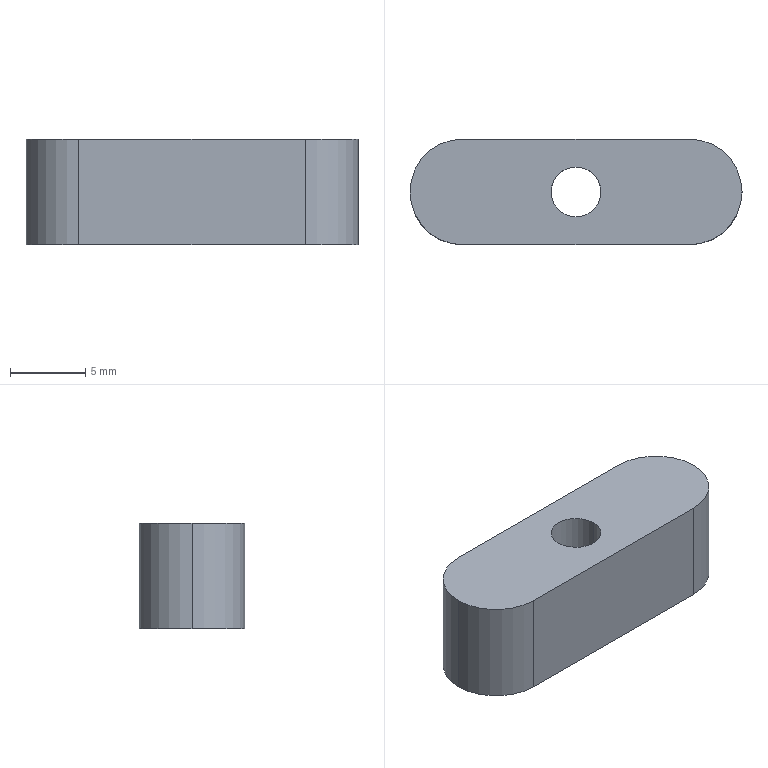Part | STEP file | BU-A13#130b | 1 solid | 9 faces | box 22 x 7 x 7 mm | volume 944.521 mm3 | cylinder 5 | plane 4 | commonest cylinder face diameters 7 x3 3.3 x2
STEP:
#1=CARTESIAN_POINT('',(0.,0.,0.));
#2=DIRECTION('',(0.,0.,1.));
#3=DIRECTION('',(1.,0.,0.));
#4=AXIS2_PLACEMENT_3D('',#1,#2,#3);
#5=CARTESIAN_POINT('',(9.15,0.,0.));
#6=VERTEX_POINT('',#5);
#7=CARTESIAN_POINT('',(9.15,0.,7.));
#8=VERTEX_POINT('',#7);
#9=CARTESIAN_POINT('',(9.15,0.,7.));
#10=DIRECTION('',(0.,0.,1.));
#11=VECTOR('',#10,1.);
#12=LINE('',#9,#11);
#13=CARTESIAN_POINT('',(7.5,0.,7.));
#14=DIRECTION('',(0.,0.,1.));
#15=DIRECTION('',(1.,0.,0.));
#16=AXIS2_PLACEMENT_3D('',#13,#14,#15);
#17=CYLINDRICAL_SURFACE('',#16,1.65);
#18=CARTESIAN_POINT('',(6.283,0.));
#19=DIRECTION('',(0.,1.));
#20=VECTOR('',#19,1.);
#21=LINE('',#18,#20);
#22=(GEOMETRIC_REPRESENTATION_CONTEXT(2)PARAMETRIC_REPRESENTATION_CONTEXT()REPRESENTATION_CONTEXT('',''));
#23=DEFINITIONAL_REPRESENTATION('',(#21),#22);
#24=PCURVE('',#17,#23);
#25=CARTESIAN_POINT('',(7.5,0.,7.));
#26=DIRECTION('',(0.,0.,1.));
#27=DIRECTION('',(1.,0.,0.));
#28=AXIS2_PLACEMENT_3D('',#25,#26,#27);
#29=CYLINDRICAL_SURFACE('',#28,1.65);
#30=CARTESIAN_POINT('',(0.,0.));
#31=DIRECTION('',(0.,1.));
#32=VECTOR('',#31,1.);
#33=LINE('',#30,#32);
#34=(GEOMETRIC_REPRESENTATION_CONTEXT(2)PARAMETRIC_REPRESENTATION_CONTEXT()REPRESENTATION_CONTEXT('',''));
#35=DEFINITIONAL_REPRESENTATION('',(#33),#34);
#36=PCURVE('',#29,#35);
#37=SURFACE_CURVE('',#12,(#24,#36),.PCURVE_S1.);
#38=EDGE_CURVE('',#6,#8,#37,.T.);
#39=ORIENTED_EDGE('',*,*,#38,.T.);
#40=CARTESIAN_POINT('',(5.85,0.,7.));
#41=VERTEX_POINT('',#40);
#42=CARTESIAN_POINT('',(7.5,0.,7.));
#43=DIRECTION('',(0.,0.,1.));
#44=DIRECTION('',(1.,0.,0.));
#45=AXIS2_PLACEMENT_3D('',#42,#43,#44);
#46=CIRCLE('',#45,1.65);
#47=CARTESIAN_POINT('',(0.,0.));
#48=DIRECTION('',(1.,0.));
#49=VECTOR('',#48,1.);
#50=LINE('',#47,#49);
#51=(GEOMETRIC_REPRESENTATION_CONTEXT(2)PARAMETRIC_REPRESENTATION_CONTEXT()REPRESENTATION_CONTEXT('',''));
#52=DEFINITIONAL_REPRESENTATION('',(#50),#51);
#53=PCURVE('',#17,#52);
#54=CARTESIAN_POINT('',(15.,0.,7.));
#55=DIRECTION('',(0.,0.,1.));
#56=DIRECTION('',(1.,0.,0.));
#57=AXIS2_PLACEMENT_3D('',#54,#55,#56);
#58=PLANE('',#57);
#59=CARTESIAN_POINT('',(-7.5,0.));
#60=DIRECTION('',(1.,0.));
#61=AXIS2_PLACEMENT_2D('',#59,#60);
#62=CIRCLE('',#61,1.65);
#63=(GEOMETRIC_REPRESENTATION_CONTEXT(2)PARAMETRIC_REPRESENTATION_CONTEXT()REPRESENTATION_CONTEXT('',''));
#64=DEFINITIONAL_REPRESENTATION('',(#62),#63);
#65=PCURVE('',#58,#64);
#66=SURFACE_CURVE('',#46,(#53,#65),.PCURVE_S1.);
#67=EDGE_CURVE('',#41,#8,#66,.T.);
#68=ORIENTED_EDGE('',*,*,#67,.F.);
#69=CARTESIAN_POINT('',(5.85,0.,0.));
#70=VERTEX_POINT('',#69);
#71=CARTESIAN_POINT('',(5.85,0.,7.));
#72=DIRECTION('',(0.,0.,1.));
#73=VECTOR('',#72,1.);
#74=LINE('',#71,#73);
#75=CARTESIAN_POINT('',(3.142,0.));
#76=DIRECTION('',(0.,1.));
#77=VECTOR('',#76,1.);
#78=LINE('',#75,#77);
#79=(GEOMETRIC_REPRESENTATION_CONTEXT(2)PARAMETRIC_REPRESENTATION_CONTEXT()REPRESENTATION_CONTEXT('',''));
#80=DEFINITIONAL_REPRESENTATION('',(#78),#79);
#81=PCURVE('',#17,#80);
#82=CARTESIAN_POINT('',(3.142,0.));
#83=DIRECTION('',(0.,1.));
#84=VECTOR('',#83,1.);
#85=LINE('',#82,#84);
#86=(GEOMETRIC_REPRESENTATION_CONTEXT(2)PARAMETRIC_REPRESENTATION_CONTEXT()REPRESENTATION_CONTEXT('',''));
#87=DEFINITIONAL_REPRESENTATION('',(#85),#86);
#88=PCURVE('',#29,#87);
#89=SURFACE_CURVE('',#74,(#81,#88),.PCURVE_S1.);
#90=EDGE_CURVE('',#70,#41,#89,.T.);
#91=ORIENTED_EDGE('',*,*,#90,.F.);
#92=CARTESIAN_POINT('',(7.5,0.,0.));
#93=DIRECTION('',(0.,0.,1.));
#94=DIRECTION('',(1.,0.,0.));
#95=AXIS2_PLACEMENT_3D('',#92,#93,#94);
#96=CIRCLE('',#95,1.65);
#97=CARTESIAN_POINT('',(0.,-7.));
#98=DIRECTION('',(1.,0.));
#99=VECTOR('',#98,1.);
#100=LINE('',#97,#99);
#101=(GEOMETRIC_REPRESENTATION_CONTEXT(2)PARAMETRIC_REPRESENTATION_CONTEXT()REPRESENTATION_CONTEXT('',''));
#102=DEFINITIONAL_REPRESENTATION('',(#100),#101);
#103=PCURVE('',#17,#102);
#104=CARTESIAN_POINT('',(15.,0.,0.));
#105=DIRECTION('',(0.,0.,1.));
#106=DIRECTION('',(1.,0.,0.));
#107=AXIS2_PLACEMENT_3D('',#104,#105,#106);
#108=PLANE('',#107);
#109=CARTESIAN_POINT('',(-7.5,0.));
#110=DIRECTION('',(1.,0.));
#111=AXIS2_PLACEMENT_2D('',#109,#110);
#112=CIRCLE('',#111,1.65);
#113=(GEOMETRIC_REPRESENTATION_CONTEXT(2)PARAMETRIC_REPRESENTATION_CONTEXT()REPRESENTATION_CONTEXT('',''));
#114=DEFINITIONAL_REPRESENTATION('',(#112),#113);
#115=PCURVE('',#108,#114);
#116=SURFACE_CURVE('',#96,(#103,#115),.PCURVE_S1.);
#117=EDGE_CURVE('',#70,#6,#116,.T.);
#118=ORIENTED_EDGE('',*,*,#117,.T.);
#119=EDGE_LOOP('',(#39,#68,#91,#118));
#120=FACE_BOUND('',#119,.F.);
#121=ADVANCED_FACE('',(#120),#17,.F.);
#122=CARTESIAN_POINT('',(-3.5,0.,7.));
#123=VERTEX_POINT('',#122);
#124=CARTESIAN_POINT('',(0.,-3.5,7.));
#125=VERTEX_POINT('',#124);
#126=CARTESIAN_POINT('',(0.,0.,7.));
#127=DIRECTION('',(0.,0.,1.));
#128=DIRECTION('',(1.,0.,0.));
#129=AXIS2_PLACEMENT_3D('',#126,#127,#128);
#130=CIRCLE('',#129,3.5);
#131=CARTESIAN_POINT('',(0.,0.,7.));
#132=DIRECTION('',(0.,0.,-1.));
#133=DIRECTION('',(-1.,0.,0.));
#134=AXIS2_PLACEMENT_3D('',#131,#132,#133);
#135=CYLINDRICAL_SURFACE('',#134,3.5);
#136=CARTESIAN_POINT('',(9.425,0.));
#137=DIRECTION('',(-1.,0.));
#138=VECTOR('',#137,1.);
#139=LINE('',#136,#138);
#140=(GEOMETRIC_REPRESENTATION_CONTEXT(2)PARAMETRIC_REPRESENTATION_CONTEXT()REPRESENTATION_CONTEXT('',''));
#141=DEFINITIONAL_REPRESENTATION('',(#139),#140);
#142=PCURVE('',#135,#141);
#143=CARTESIAN_POINT('',(-15.,0.));
#144=DIRECTION('',(1.,0.));
#145=AXIS2_PLACEMENT_2D('',#143,#144);
#146=CIRCLE('',#145,3.5);
#147=(GEOMETRIC_REPRESENTATION_CONTEXT(2)PARAMETRIC_REPRESENTATION_CONTEXT()REPRESENTATION_CONTEXT('',''));
#148=DEFINITIONAL_REPRESENTATION('',(#146),#147);
#149=PCURVE('',#58,#148);
#150=SURFACE_CURVE('',#130,(#142,#149),.PCURVE_S1.);
#151=EDGE_CURVE('',#123,#125,#150,.T.);
#152=ORIENTED_EDGE('',*,*,#151,.F.);
#153=CARTESIAN_POINT('',(-3.5,0.,0.));
#154=VERTEX_POINT('',#153);
#155=CARTESIAN_POINT('',(-3.5,0.,7.));
#156=DIRECTION('',(0.,0.,-1.));
#157=VECTOR('',#156,1.);
#158=LINE('',#155,#157);
#159=CARTESIAN_POINT('',(6.283,0.));
#160=DIRECTION('',(0.,1.));
#161=VECTOR('',#160,1.);
#162=LINE('',#159,#161);
#163=(GEOMETRIC_REPRESENTATION_CONTEXT(2)PARAMETRIC_REPRESENTATION_CONTEXT()REPRESENTATION_CONTEXT('',''));
#164=DEFINITIONAL_REPRESENTATION('',(#162),#163);
#165=PCURVE('',#135,#164);
#166=CARTESIAN_POINT('',(0.,0.,7.));
#167=DIRECTION('',(0.,0.,-1.));
#168=DIRECTION('',(-1.,0.,0.));
#169=AXIS2_PLACEMENT_3D('',#166,#167,#168);
#170=CYLINDRICAL_SURFACE('',#169,3.5);
#171=CARTESIAN_POINT('',(0.,0.));
#172=DIRECTION('',(0.,1.));
#173=VECTOR('',#172,1.);
#174=LINE('',#171,#173);
#175=(GEOMETRIC_REPRESENTATION_CONTEXT(2)PARAMETRIC_REPRESENTATION_CONTEXT()REPRESENTATION_CONTEXT('',''));
#176=DEFINITIONAL_REPRESENTATION('',(#174),#175);
#177=PCURVE('',#170,#176);
#178=SURFACE_CURVE('',#158,(#165,#177),.PCURVE_S1.);
#179=EDGE_CURVE('',#123,#154,#178,.T.);
#180=ORIENTED_EDGE('',*,*,#179,.T.);
#181=CARTESIAN_POINT('',(0.,-3.5,0.));
#182=VERTEX_POINT('',#181);
#183=CARTESIAN_POINT('',(0.,0.,0.));
#184=DIRECTION('',(0.,0.,1.));
#185=DIRECTION('',(1.,0.,0.));
#186=AXIS2_PLACEMENT_3D('',#183,#184,#185);
#187=CIRCLE('',#186,3.5);
#188=CARTESIAN_POINT('',(9.425,7.));
#189=DIRECTION('',(-1.,0.));
#190=VECTOR('',#189,1.);
#191=LINE('',#188,#190);
#192=(GEOMETRIC_REPRESENTATION_CONTEXT(2)PARAMETRIC_REPRESENTATION_CONTEXT()REPRESENTATION_CONTEXT('',''));
#193=DEFINITIONAL_REPRESENTATION('',(#191),#192);
#194=PCURVE('',#135,#193);
#195=CARTESIAN_POINT('',(-15.,0.));
#196=DIRECTION('',(1.,0.));
#197=AXIS2_PLACEMENT_2D('',#195,#196);
#198=CIRCLE('',#197,3.5);
#199=(GEOMETRIC_REPRESENTATION_CONTEXT(2)PARAMETRIC_REPRESENTATION_CONTEXT()REPRESENTATION_CONTEXT('',''));
#200=DEFINITIONAL_REPRESENTATION('',(#198),#199);
#201=PCURVE('',#108,#200);
#202=SURFACE_CURVE('',#187,(#194,#201),.PCURVE_S1.);
#203=EDGE_CURVE('',#154,#182,#202,.T.);
#204=ORIENTED_EDGE('',*,*,#203,.T.);
#205=CARTESIAN_POINT('',(0.,-3.5,7.));
#206=DIRECTION('',(0.,0.,-1.));
#207=VECTOR('',#206,1.);
#208=LINE('',#205,#207);
#209=CARTESIAN_POINT('',(4.712,0.));
#210=DIRECTION('',(0.,1.));
#211=VECTOR('',#210,1.);
#212=LINE('',#209,#211);
#213=(GEOMETRIC_REPRESENTATION_CONTEXT(2)PARAMETRIC_REPRESENTATION_CONTEXT()REPRESENTATION_CONTEXT('',''));
#214=DEFINITIONAL_REPRESENTATION('',(#212),#213);
#215=PCURVE('',#135,#214);
#216=CARTESIAN_POINT('',(0.,-3.5,7.));
#217=DIRECTION('',(0.,1.,0.));
#218=DIRECTION('',(0.,0.,1.));
#219=AXIS2_PLACEMENT_3D('',#216,#217,#218);
#220=PLANE('',#219);
#221=CARTESIAN_POINT('',(0.,0.));
#222=DIRECTION('',(-1.,0.));
#223=VECTOR('',#222,1.);
#224=LINE('',#221,#223);
#225=(GEOMETRIC_REPRESENTATION_CONTEXT(2)PARAMETRIC_REPRESENTATION_CONTEXT()REPRESENTATION_CONTEXT('',''));
#226=DEFINITIONAL_REPRESENTATION('',(#224),#225);
#227=PCURVE('',#220,#226);
#228=SURFACE_CURVE('',#208,(#215,#227),.PCURVE_S1.);
#229=EDGE_CURVE('',#125,#182,#228,.T.);
#230=ORIENTED_EDGE('',*,*,#229,.F.);
#231=EDGE_LOOP('',(#152,#180,#204,#230));
#232=FACE_BOUND('',#231,.T.);
#233=ADVANCED_FACE('',(#232),#135,.T.);
#234=CARTESIAN_POINT('',(15.,-3.5,0.));
#235=VERTEX_POINT('',#234);
#236=CARTESIAN_POINT('',(15.,3.5,0.));
#237=VERTEX_POINT('',#236);
#238=CARTESIAN_POINT('',(15.,0.,0.));
#239=DIRECTION('',(0.,0.,1.));
#240=DIRECTION('',(1.,0.,0.));
#241=AXIS2_PLACEMENT_3D('',#238,#239,#240);
#242=CIRCLE('',#241,3.5);
#243=CARTESIAN_POINT('',(15.,0.,7.));
#244=DIRECTION('',(0.,0.,-1.));
#245=DIRECTION('',(-1.,0.,0.));
#246=AXIS2_PLACEMENT_3D('',#243,#244,#245);
#247=CYLINDRICAL_SURFACE('',#246,3.5);
#248=CARTESIAN_POINT('',(9.425,7.));
#249=DIRECTION('',(-1.,0.));
#250=VECTOR('',#249,1.);
#251=LINE('',#248,#250);
#252=(GEOMETRIC_REPRESENTATION_CONTEXT(2)PARAMETRIC_REPRESENTATION_CONTEXT()REPRESENTATION_CONTEXT('',''));
#253=DEFINITIONAL_REPRESENTATION('',(#251),#252);
#254=PCURVE('',#247,#253);
#255=CARTESIAN_POINT('',(0.,0.));
#256=DIRECTION('',(1.,0.));
#257=AXIS2_PLACEMENT_2D('',#255,#256);
#258=CIRCLE('',#257,3.5);
#259=(GEOMETRIC_REPRESENTATION_CONTEXT(2)PARAMETRIC_REPRESENTATION_CONTEXT()REPRESENTATION_CONTEXT('',''));
#260=DEFINITIONAL_REPRESENTATION('',(#258),#259);
#261=PCURVE('',#108,#260);
#262=SURFACE_CURVE('',#242,(#254,#261),.PCURVE_S1.);
#263=EDGE_CURVE('',#235,#237,#262,.T.);
#264=ORIENTED_EDGE('',*,*,#263,.T.);
#265=CARTESIAN_POINT('',(15.,3.5,7.));
#266=VERTEX_POINT('',#265);
#267=CARTESIAN_POINT('',(15.,3.5,7.));
#268=DIRECTION('',(0.,0.,-1.));
#269=VECTOR('',#268,1.);
#270=LINE('',#267,#269);
#271=CARTESIAN_POINT('',(1.571,0.));
#272=DIRECTION('',(0.,1.));
#273=VECTOR('',#272,1.);
#274=LINE('',#271,#273);
#275=(GEOMETRIC_REPRESENTATION_CONTEXT(2)PARAMETRIC_REPRESENTATION_CONTEXT()REPRESENTATION_CONTEXT('',''));
#276=DEFINITIONAL_REPRESENTATION('',(#274),#275);
#277=PCURVE('',#247,#276);
#278=CARTESIAN_POINT('',(15.,3.5,7.));
#279=DIRECTION('',(0.,-1.,0.));
#280=DIRECTION('',(0.,0.,-1.));
#281=AXIS2_PLACEMENT_3D('',#278,#279,#280);
#282=PLANE('',#281);
#283=CARTESIAN_POINT('',(0.,0.));
#284=DIRECTION('',(1.,0.));
#285=VECTOR('',#284,1.);
#286=LINE('',#283,#285);
#287=(GEOMETRIC_REPRESENTATION_CONTEXT(2)PARAMETRIC_REPRESENTATION_CONTEXT()REPRESENTATION_CONTEXT('',''));
#288=DEFINITIONAL_REPRESENTATION('',(#286),#287);
#289=PCURVE('',#282,#288);
#290=SURFACE_CURVE('',#270,(#277,#289),.PCURVE_S1.);
#291=EDGE_CURVE('',#266,#237,#290,.T.);
#292=ORIENTED_EDGE('',*,*,#291,.F.);
#293=CARTESIAN_POINT('',(15.,-3.5,7.));
#294=VERTEX_POINT('',#293);
#295=CARTESIAN_POINT('',(15.,0.,7.));
#296=DIRECTION('',(0.,0.,1.));
#297=DIRECTION('',(1.,0.,0.));
#298=AXIS2_PLACEMENT_3D('',#295,#296,#297);
#299=CIRCLE('',#298,3.5);
#300=CARTESIAN_POINT('',(9.425,0.));
#301=DIRECTION('',(-1.,0.));
#302=VECTOR('',#301,1.);
#303=LINE('',#300,#302);
#304=(GEOMETRIC_REPRESENTATION_CONTEXT(2)PARAMETRIC_REPRESENTATION_CONTEXT()REPRESENTATION_CONTEXT('',''));
#305=DEFINITIONAL_REPRESENTATION('',(#303),#304);
#306=PCURVE('',#247,#305);
#307=CARTESIAN_POINT('',(0.,0.));
#308=DIRECTION('',(1.,0.));
#309=AXIS2_PLACEMENT_2D('',#307,#308);
#310=CIRCLE('',#309,3.5);
#311=(GEOMETRIC_REPRESENTATION_CONTEXT(2)PARAMETRIC_REPRESENTATION_CONTEXT()REPRESENTATION_CONTEXT('',''));
#312=DEFINITIONAL_REPRESENTATION('',(#310),#311);
#313=PCURVE('',#58,#312);
#314=SURFACE_CURVE('',#299,(#306,#313),.PCURVE_S1.);
#315=EDGE_CURVE('',#294,#266,#314,.T.);
#316=ORIENTED_EDGE('',*,*,#315,.F.);
#317=CARTESIAN_POINT('',(15.,-3.5,7.));
#318=DIRECTION('',(0.,0.,-1.));
#319=VECTOR('',#318,1.);
#320=LINE('',#317,#319);
#321=CARTESIAN_POINT('',(4.712,0.));
#322=DIRECTION('',(0.,1.));
#323=VECTOR('',#322,1.);
#324=LINE('',#321,#323);
#325=(GEOMETRIC_REPRESENTATION_CONTEXT(2)PARAMETRIC_REPRESENTATION_CONTEXT()REPRESENTATION_CONTEXT('',''));
#326=DEFINITIONAL_REPRESENTATION('',(#324),#325);
#327=PCURVE('',#247,#326);
#328=CARTESIAN_POINT('',(0.,15.));
#329=DIRECTION('',(-1.,0.));
#330=VECTOR('',#329,1.);
#331=LINE('',#328,#330);
#332=(GEOMETRIC_REPRESENTATION_CONTEXT(2)PARAMETRIC_REPRESENTATION_CONTEXT()REPRESENTATION_CONTEXT('',''));
#333=DEFINITIONAL_REPRESENTATION('',(#331),#332);
#334=PCURVE('',#220,#333);
#335=SURFACE_CURVE('',#320,(#327,#334),.PCURVE_S1.);
#336=EDGE_CURVE('',#294,#235,#335,.T.);
#337=ORIENTED_EDGE('',*,*,#336,.T.);
#338=EDGE_LOOP('',(#264,#292,#316,#337));
#339=FACE_BOUND('',#338,.T.);
#340=ADVANCED_FACE('',(#339),#247,.T.);
#341=CARTESIAN_POINT('',(0.,3.5,0.));
#342=VERTEX_POINT('',#341);
#343=CARTESIAN_POINT('',(15.,3.5,0.));
#344=DIRECTION('',(-1.,0.,0.));
#345=VECTOR('',#344,1.);
#346=LINE('',#343,#345);
#347=CARTESIAN_POINT('',(7.,0.));
#348=DIRECTION('',(0.,-1.));
#349=VECTOR('',#348,1.);
#350=LINE('',#347,#349);
#351=(GEOMETRIC_REPRESENTATION_CONTEXT(2)PARAMETRIC_REPRESENTATION_CONTEXT()REPRESENTATION_CONTEXT('',''));
#352=DEFINITIONAL_REPRESENTATION('',(#350),#351);
#353=PCURVE('',#282,#352);
#354=CARTESIAN_POINT('',(0.,3.5));
#355=DIRECTION('',(-1.,0.));
#356=VECTOR('',#355,1.);
#357=LINE('',#354,#356);
#358=(GEOMETRIC_REPRESENTATION_CONTEXT(2)PARAMETRIC_REPRESENTATION_CONTEXT()REPRESENTATION_CONTEXT('',''));
#359=DEFINITIONAL_REPRESENTATION('',(#357),#358);
#360=PCURVE('',#108,#359);
#361=SURFACE_CURVE('',#346,(#353,#360),.PCURVE_S1.);
#362=EDGE_CURVE('',#237,#342,#361,.T.);
#363=ORIENTED_EDGE('',*,*,#362,.T.);
#364=CARTESIAN_POINT('',(0.,3.5,7.));
#365=VERTEX_POINT('',#364);
#366=CARTESIAN_POINT('',(0.,3.5,7.));
#367=DIRECTION('',(0.,0.,-1.));
#368=VECTOR('',#367,1.);
#369=LINE('',#366,#368);
#370=CARTESIAN_POINT('',(0.,-15.));
#371=DIRECTION('',(1.,0.));
#372=VECTOR('',#371,1.);
#373=LINE('',#370,#372);
#374=(GEOMETRIC_REPRESENTATION_CONTEXT(2)PARAMETRIC_REPRESENTATION_CONTEXT()REPRESENTATION_CONTEXT('',''));
#375=DEFINITIONAL_REPRESENTATION('',(#373),#374);
#376=PCURVE('',#282,#375);
#377=CARTESIAN_POINT('',(1.571,0.));
#378=DIRECTION('',(0.,1.));
#379=VECTOR('',#378,1.);
#380=LINE('',#377,#379);
#381=(GEOMETRIC_REPRESENTATION_CONTEXT(2)PARAMETRIC_REPRESENTATION_CONTEXT()REPRESENTATION_CONTEXT('',''));
#382=DEFINITIONAL_REPRESENTATION('',(#380),#381);
#383=PCURVE('',#170,#382);
#384=SURFACE_CURVE('',#369,(#376,#383),.PCURVE_S1.);
#385=EDGE_CURVE('',#365,#342,#384,.T.);
#386=ORIENTED_EDGE('',*,*,#385,.F.);
#387=CARTESIAN_POINT('',(15.,3.5,7.));
#388=DIRECTION('',(-1.,0.,0.));
#389=VECTOR('',#388,1.);
#390=LINE('',#387,#389);
#391=CARTESIAN_POINT('',(0.,0.));
#392=DIRECTION('',(0.,-1.));
#393=VECTOR('',#392,1.);
#394=LINE('',#391,#393);
#395=(GEOMETRIC_REPRESENTATION_CONTEXT(2)PARAMETRIC_REPRESENTATION_CONTEXT()REPRESENTATION_CONTEXT('',''));
#396=DEFINITIONAL_REPRESENTATION('',(#394),#395);
#397=PCURVE('',#282,#396);
#398=CARTESIAN_POINT('',(0.,3.5));
#399=DIRECTION('',(-1.,0.));
#400=VECTOR('',#399,1.);
#401=LINE('',#398,#400);
#402=(GEOMETRIC_REPRESENTATION_CONTEXT(2)PARAMETRIC_REPRESENTATION_CONTEXT()REPRESENTATION_CONTEXT('',''));
#403=DEFINITIONAL_REPRESENTATION('',(#401),#402);
#404=PCURVE('',#58,#403);
#405=SURFACE_CURVE('',#390,(#397,#404),.PCURVE_S1.);
#406=EDGE_CURVE('',#266,#365,#405,.T.);
#407=ORIENTED_EDGE('',*,*,#406,.F.);
#408=ORIENTED_EDGE('',*,*,#291,.T.);
#409=EDGE_LOOP('',(#363,#386,#407,#408));
#410=FACE_BOUND('',#409,.T.);
#411=ADVANCED_FACE('',(#410),#282,.F.);
#412=ORIENTED_EDGE('',*,*,#179,.F.);
#413=CARTESIAN_POINT('',(0.,0.,7.));
#414=DIRECTION('',(0.,0.,1.));
#415=DIRECTION('',(1.,0.,0.));
#416=AXIS2_PLACEMENT_3D('',#413,#414,#415);
#417=CIRCLE('',#416,3.5);
#418=CARTESIAN_POINT('',(3.142,0.));
#419=DIRECTION('',(-1.,0.));
#420=VECTOR('',#419,1.);
#421=LINE('',#418,#420);
#422=(GEOMETRIC_REPRESENTATION_CONTEXT(2)PARAMETRIC_REPRESENTATION_CONTEXT()REPRESENTATION_CONTEXT('',''));
#423=DEFINITIONAL_REPRESENTATION('',(#421),#422);
#424=PCURVE('',#170,#423);
#425=CARTESIAN_POINT('',(-15.,0.));
#426=DIRECTION('',(1.,0.));
#427=AXIS2_PLACEMENT_2D('',#425,#426);
#428=CIRCLE('',#427,3.5);
#429=(GEOMETRIC_REPRESENTATION_CONTEXT(2)PARAMETRIC_REPRESENTATION_CONTEXT()REPRESENTATION_CONTEXT('',''));
#430=DEFINITIONAL_REPRESENTATION('',(#428),#429);
#431=PCURVE('',#58,#430);
#432=SURFACE_CURVE('',#417,(#424,#431),.PCURVE_S1.);
#433=EDGE_CURVE('',#365,#123,#432,.T.);
#434=ORIENTED_EDGE('',*,*,#433,.F.);
#435=ORIENTED_EDGE('',*,*,#385,.T.);
#436=CARTESIAN_POINT('',(0.,0.,0.));
#437=DIRECTION('',(0.,0.,1.));
#438=DIRECTION('',(1.,0.,0.));
#439=AXIS2_PLACEMENT_3D('',#436,#437,#438);
#440=CIRCLE('',#439,3.5);
#441=CARTESIAN_POINT('',(3.142,7.));
#442=DIRECTION('',(-1.,0.));
#443=VECTOR('',#442,1.);
#444=LINE('',#441,#443);
#445=(GEOMETRIC_REPRESENTATION_CONTEXT(2)PARAMETRIC_REPRESENTATION_CONTEXT()REPRESENTATION_CONTEXT('',''));
#446=DEFINITIONAL_REPRESENTATION('',(#444),#445);
#447=PCURVE('',#170,#446);
#448=CARTESIAN_POINT('',(-15.,0.));
#449=DIRECTION('',(1.,0.));
#450=AXIS2_PLACEMENT_2D('',#448,#449);
#451=CIRCLE('',#450,3.5);
#452=(GEOMETRIC_REPRESENTATION_CONTEXT(2)PARAMETRIC_REPRESENTATION_CONTEXT()REPRESENTATION_CONTEXT('',''));
#453=DEFINITIONAL_REPRESENTATION('',(#451),#452);
#454=PCURVE('',#108,#453);
#455=SURFACE_CURVE('',#440,(#447,#454),.PCURVE_S1.);
#456=EDGE_CURVE('',#342,#154,#455,.T.);
#457=ORIENTED_EDGE('',*,*,#456,.T.);
#458=EDGE_LOOP('',(#412,#434,#435,#457));
#459=FACE_BOUND('',#458,.T.);
#460=ADVANCED_FACE('',(#459),#170,.T.);
#461=CARTESIAN_POINT('',(0.,-3.5,0.));
#462=DIRECTION('',(1.,0.,0.));
#463=VECTOR('',#462,1.);
#464=LINE('',#461,#463);
#465=CARTESIAN_POINT('',(-7.,0.));
#466=DIRECTION('',(0.,1.));
#467=VECTOR('',#466,1.);
#468=LINE('',#465,#467);
#469=(GEOMETRIC_REPRESENTATION_CONTEXT(2)PARAMETRIC_REPRESENTATION_CONTEXT()REPRESENTATION_CONTEXT('',''));
#470=DEFINITIONAL_REPRESENTATION('',(#468),#469);
#471=PCURVE('',#220,#470);
#472=CARTESIAN_POINT('',(-15.,-3.5));
#473=DIRECTION('',(1.,0.));
#474=VECTOR('',#473,1.);
#475=LINE('',#472,#474);
#476=(GEOMETRIC_REPRESENTATION_CONTEXT(2)PARAMETRIC_REPRESENTATION_CONTEXT()REPRESENTATION_CONTEXT('',''));
#477=DEFINITIONAL_REPRESENTATION('',(#475),#476);
#478=PCURVE('',#108,#477);
#479=SURFACE_CURVE('',#464,(#471,#478),.PCURVE_S1.);
#480=EDGE_CURVE('',#182,#235,#479,.T.);
#481=ORIENTED_EDGE('',*,*,#480,.T.);
#482=ORIENTED_EDGE('',*,*,#336,.F.);
#483=CARTESIAN_POINT('',(0.,-3.5,7.));
#484=DIRECTION('',(1.,0.,0.));
#485=VECTOR('',#484,1.);
#486=LINE('',#483,#485);
#487=CARTESIAN_POINT('',(0.,0.));
#488=DIRECTION('',(0.,1.));
#489=VECTOR('',#488,1.);
#490=LINE('',#487,#489);
#491=(GEOMETRIC_REPRESENTATION_CONTEXT(2)PARAMETRIC_REPRESENTATION_CONTEXT()REPRESENTATION_CONTEXT('',''));
#492=DEFINITIONAL_REPRESENTATION('',(#490),#491);
#493=PCURVE('',#220,#492);
#494=CARTESIAN_POINT('',(-15.,-3.5));
#495=DIRECTION('',(1.,0.));
#496=VECTOR('',#495,1.);
#497=LINE('',#494,#496);
#498=(GEOMETRIC_REPRESENTATION_CONTEXT(2)PARAMETRIC_REPRESENTATION_CONTEXT()REPRESENTATION_CONTEXT('',''));
#499=DEFINITIONAL_REPRESENTATION('',(#497),#498);
#500=PCURVE('',#58,#499);
#501=SURFACE_CURVE('',#486,(#493,#500),.PCURVE_S1.);
#502=EDGE_CURVE('',#125,#294,#501,.T.);
#503=ORIENTED_EDGE('',*,*,#502,.F.);
#504=ORIENTED_EDGE('',*,*,#229,.T.);
#505=EDGE_LOOP('',(#481,#482,#503,#504));
#506=FACE_BOUND('',#505,.T.);
#507=ADVANCED_FACE('',(#506),#220,.F.);
#508=CARTESIAN_POINT('',(7.5,0.,7.));
#509=DIRECTION('',(0.,0.,1.));
#510=DIRECTION('',(1.,0.,0.));
#511=AXIS2_PLACEMENT_3D('',#508,#509,#510);
#512=CIRCLE('',#511,1.65);
#513=CARTESIAN_POINT('',(-7.5,0.));
#514=DIRECTION('',(1.,0.));
#515=AXIS2_PLACEMENT_2D('',#513,#514);
#516=CIRCLE('',#515,1.65);
#517=(GEOMETRIC_REPRESENTATION_CONTEXT(2)PARAMETRIC_REPRESENTATION_CONTEXT()REPRESENTATION_CONTEXT('',''));
#518=DEFINITIONAL_REPRESENTATION('',(#516),#517);
#519=PCURVE('',#58,#518);
#520=CARTESIAN_POINT('',(0.,0.));
#521=DIRECTION('',(1.,0.));
#522=VECTOR('',#521,1.);
#523=LINE('',#520,#522);
#524=(GEOMETRIC_REPRESENTATION_CONTEXT(2)PARAMETRIC_REPRESENTATION_CONTEXT()REPRESENTATION_CONTEXT('',''));
#525=DEFINITIONAL_REPRESENTATION('',(#523),#524);
#526=PCURVE('',#29,#525);
#527=SURFACE_CURVE('',#512,(#519,#526),.PCURVE_S1.);
#528=EDGE_CURVE('',#8,#41,#527,.T.);
#529=ORIENTED_EDGE('',*,*,#528,.F.);
#530=ORIENTED_EDGE('',*,*,#67,.F.);
#531=EDGE_LOOP('',(#529,#530));
#532=FACE_BOUND('',#531,.T.);
#533=ORIENTED_EDGE('',*,*,#315,.T.);
#534=ORIENTED_EDGE('',*,*,#406,.T.);
#535=ORIENTED_EDGE('',*,*,#433,.T.);
#536=ORIENTED_EDGE('',*,*,#151,.T.);
#537=ORIENTED_EDGE('',*,*,#502,.T.);
#538=EDGE_LOOP('',(#533,#534,#535,#536,#537));
#539=FACE_BOUND('',#538,.T.);
#540=ADVANCED_FACE('',(#532,#539),#58,.T.);
#541=CARTESIAN_POINT('',(7.5,0.,0.));
#542=DIRECTION('',(0.,0.,1.));
#543=DIRECTION('',(1.,0.,0.));
#544=AXIS2_PLACEMENT_3D('',#541,#542,#543);
#545=CIRCLE('',#544,1.65);
#546=CARTESIAN_POINT('',(-7.5,0.));
#547=DIRECTION('',(1.,0.));
#548=AXIS2_PLACEMENT_2D('',#546,#547);
#549=CIRCLE('',#548,1.65);
#550=(GEOMETRIC_REPRESENTATION_CONTEXT(2)PARAMETRIC_REPRESENTATION_CONTEXT()REPRESENTATION_CONTEXT('',''));
#551=DEFINITIONAL_REPRESENTATION('',(#549),#550);
#552=PCURVE('',#108,#551);
#553=CARTESIAN_POINT('',(0.,-7.));
#554=DIRECTION('',(1.,0.));
#555=VECTOR('',#554,1.);
#556=LINE('',#553,#555);
#557=(GEOMETRIC_REPRESENTATION_CONTEXT(2)PARAMETRIC_REPRESENTATION_CONTEXT()REPRESENTATION_CONTEXT('',''));
#558=DEFINITIONAL_REPRESENTATION('',(#556),#557);
#559=PCURVE('',#29,#558);
#560=SURFACE_CURVE('',#545,(#552,#559),.PCURVE_S1.);
#561=EDGE_CURVE('',#6,#70,#560,.T.);
#562=ORIENTED_EDGE('',*,*,#561,.T.);
#563=ORIENTED_EDGE('',*,*,#117,.T.);
#564=EDGE_LOOP('',(#562,#563));
#565=FACE_BOUND('',#564,.T.);
#566=ORIENTED_EDGE('',*,*,#263,.F.);
#567=ORIENTED_EDGE('',*,*,#480,.F.);
#568=ORIENTED_EDGE('',*,*,#203,.F.);
#569=ORIENTED_EDGE('',*,*,#456,.F.);
#570=ORIENTED_EDGE('',*,*,#362,.F.);
#571=EDGE_LOOP('',(#566,#567,#568,#569,#570));
#572=FACE_BOUND('',#571,.T.);
#573=ADVANCED_FACE('',(#565,#572),#108,.F.);
#574=ORIENTED_EDGE('',*,*,#528,.F.);
#575=ORIENTED_EDGE('',*,*,#38,.F.);
#576=ORIENTED_EDGE('',*,*,#561,.T.);
#577=ORIENTED_EDGE('',*,*,#90,.T.);
#578=EDGE_LOOP('',(#574,#575,#576,#577));
#579=FACE_BOUND('',#578,.F.);
#580=ADVANCED_FACE('',(#579),#29,.F.);
#581=CLOSED_SHELL('',(#121,#233,#340,#411,#460,#507,#540,#573,#580));
#582=MANIFOLD_SOLID_BREP('',#581);
#583=(LENGTH_UNIT()NAMED_UNIT(*)SI_UNIT(.MILLI.,.METRE.));
#584=UNCERTAINTY_MEASURE_WITH_UNIT(LENGTH_MEASURE(0.0000001),#583,'','');
#585=(NAMED_UNIT(*)PLANE_ANGLE_UNIT()SI_UNIT($,.RADIAN.));
#586=(NAMED_UNIT(*)SI_UNIT($,.STERADIAN.)SOLID_ANGLE_UNIT());
#587=(GEOMETRIC_REPRESENTATION_CONTEXT(3)GLOBAL_UNCERTAINTY_ASSIGNED_CONTEXT((#584))GLOBAL_UNIT_ASSIGNED_CONTEXT((#583,#585,#586))REPRESENTATION_CONTEXT('',''));
#588=ADVANCED_BREP_SHAPE_REPRESENTATION('',(#4,#582),#587);